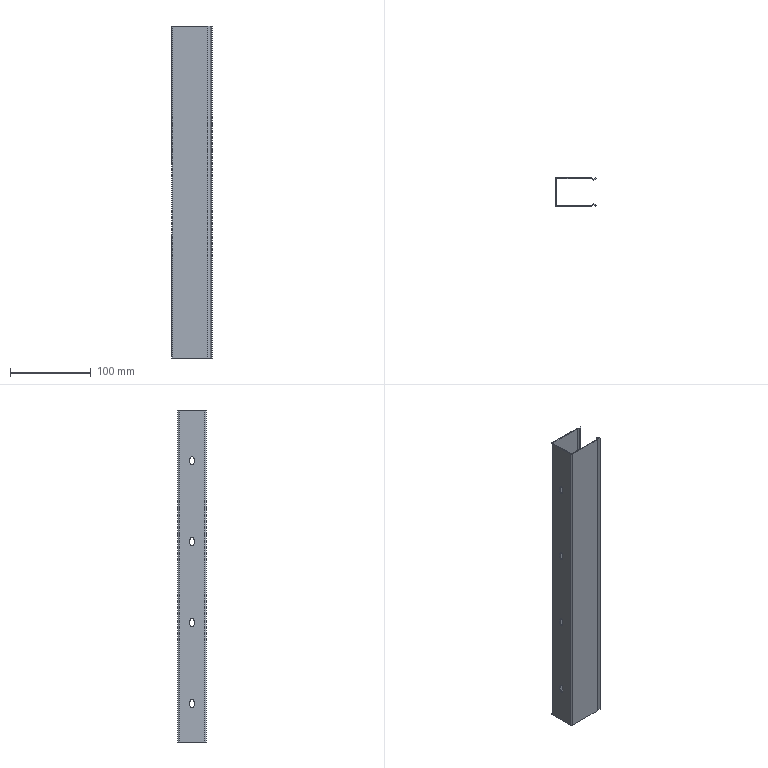Part | STEP file | 35 wire duct_410 | 1 solid | 42 faces | box 50.625 x 35 x 410 mm | volume 55518 mm3 | plane 26 | cylinder 16 | commonest cylinder face diameters 5 x12 1 x2 3 x2